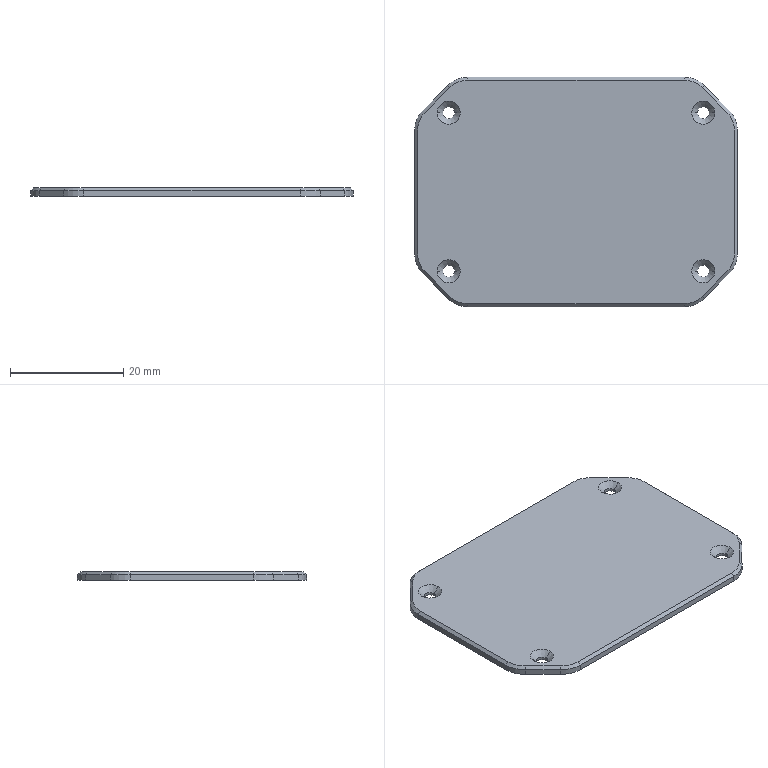NC program | NX | posted with a generic post | part box 57 x 40.5 x 1.5 mm
Lines 1 to 1491 of 7802:
N10 G17 G21 G94 G90
(PLANAR_PROFILE , TOOL : D4)
N12 T01 M6
N14 G54
N16 G17 G0 G90 X2.1 Y31.609 S6500 M3
N18 G43 Z20. H1
N20 Z0.1
N22 G94 G1 Y8.668 Z0.06 F1200.
N24 X1.827 Y7.266 Z0.057
N26 X1.281 Y5.947 Z0.055
N28 X0.482 Y4.763 Z0.052
N30 X-4.763 Y-0.482 Z0.04
N32 X-5.947 Y-1.281 Z0.037
N34 X-7.266 Y-1.827 Z0.035
N36 X-8.668 Y-2.1 Z0.032
N38 X-48.332 Z-0.037
N40 X-49.734 Y-1.827 Z-0.04
N42 X-51.053 Y-1.281 Z-0.042
N44 X-52.237 Y-0.482 Z-0.045
N46 X-57.482 Y4.763 Z-0.058
N48 X-58.281 Y5.947 Z-0.06
N50 X-58.827 Y7.266 Z-0.063
N52 X-59.1 Y8.668 Z-0.065
N54 Y31.832 Z-0.106
N56 X-58.827 Y33.234 Z-0.108
N58 X-58.281 Y34.553 Z-0.11
N60 X-57.482 Y35.737 Z-0.113
N62 X-52.237 Y40.982 Z-0.126
N64 X-51.053 Y41.781 Z-0.128
N66 X-49.734 Y42.327 Z-0.131
N68 X-48.332 Y42.6 Z-0.133
N70 X-8.668 Z-0.203
N72 X-7.266 Y42.327 Z-0.205
N74 X-5.947 Y41.781 Z-0.208
N76 X-4.763 Y40.982 Z-0.21
N78 X0.482 Y35.737 Z-0.223
N80 X1.281 Y34.553 Z-0.226
N82 X1.827 Y33.234 Z-0.228
N84 X2.1 Y31.832 Z-0.231
N86 Y8.668 Z-0.271
N88 X1.827 Y7.266 Z-0.273
N90 X1.281 Y5.947 Z-0.276
N92 X0.482 Y4.763 Z-0.278
N94 X-4.763 Y-0.482 Z-0.291
N96 X-5.947 Y-1.281 Z-0.294
N98 X-7.266 Y-1.827 Z-0.296
N100 X-8.668 Y-2.1 Z-0.299
N102 X-9.321 Z-0.3
N104 X-47.679 F2000.
N106 G2 X-52.699 Y-0.02 R7.1
N108 G1 X-57.02 Y4.301
N110 G2 X-59.1 Y9.321 R7.1
N112 G1 Y31.179
N114 G2 X-57.02 Y36.199 R7.1
N116 G1 X-52.699 Y40.52
N118 G2 X-47.679 Y42.6 R7.1
N120 G1 X-9.321
N122 G2 X-4.301 Y40.52 R7.1
N124 G1 X0.02 Y36.199
N126 G2 X2.1 Y31.179 R7.1
N128 G1 Y9.321
N130 G2 X0.02 Y4.301 R7.1
N132 G1 X-4.301 Y-0.02
N134 G2 X-9.321 Y-2.1 R7.1
N136 G1 Z-0.2
N138 G0 Z20.
N140 X2.1 Y31.609
N142 Z-0.2
N144 G1 Y8.668 Z-0.24 F1200.
N146 X1.827 Y7.266 Z-0.243
N148 X1.281 Y5.947 Z-0.245
N150 X0.482 Y4.763 Z-0.248
N152 X-4.763 Y-0.482 Z-0.26
N154 X-5.947 Y-1.281 Z-0.263
N156 X-7.266 Y-1.827 Z-0.265
N158 X-8.668 Y-2.1 Z-0.268
N160 X-48.332 Z-0.337
N162 X-49.734 Y-1.827 Z-0.34
N164 X-51.053 Y-1.281 Z-0.342
N166 X-52.237 Y-0.482 Z-0.345
N168 X-57.482 Y4.763 Z-0.358
N170 X-58.281 Y5.947 Z-0.36
N172 X-58.827 Y7.266 Z-0.363
N174 X-59.1 Y8.668 Z-0.365
N176 Y31.832 Z-0.406
N178 X-58.827 Y33.234 Z-0.408
N180 X-58.281 Y34.553 Z-0.41
N182 X-57.482 Y35.737 Z-0.413
N184 X-52.237 Y40.982 Z-0.426
N186 X-51.053 Y41.781 Z-0.428
N188 X-49.734 Y42.327 Z-0.431
N190 X-48.332 Y42.6 Z-0.433
N192 X-8.668 Z-0.503
N194 X-7.266 Y42.327 Z-0.505
N196 X-5.947 Y41.781 Z-0.508
N198 X-4.763 Y40.982 Z-0.51
N200 X0.482 Y35.737 Z-0.523
N202 X1.281 Y34.553 Z-0.526
N204 X1.827 Y33.234 Z-0.528
N206 X2.1 Y31.832 Z-0.531
N208 Y8.668 Z-0.571
N210 X1.827 Y7.266 Z-0.573
N212 X1.281 Y5.947 Z-0.576
N214 X0.482 Y4.763 Z-0.578
N216 X-4.763 Y-0.482 Z-0.591
N218 X-5.947 Y-1.281 Z-0.594
N220 X-7.266 Y-1.827 Z-0.596
N222 X-8.668 Y-2.1 Z-0.599
N224 X-9.321 Z-0.6
N226 X-47.679 F2000.
N228 G2 X-52.699 Y-0.02 R7.1
N230 G1 X-57.02 Y4.301
N232 G2 X-59.1 Y9.321 R7.1
N234 G1 Y31.179
N236 G2 X-57.02 Y36.199 R7.1
N238 G1 X-52.699 Y40.52
N240 G2 X-47.679 Y42.6 R7.1
N242 G1 X-9.321
N244 G2 X-4.301 Y40.52 R7.1
N246 G1 X0.02 Y36.199
N248 G2 X2.1 Y31.179 R7.1
N250 G1 Y9.321
N252 G2 X0.02 Y4.301 R7.1
N254 G1 X-4.301 Y-0.02
N256 G2 X-9.321 Y-2.1 R7.1
N258 G1 Z-0.5
N260 G0 Z20.
N262 X2.1 Y31.609
N264 Z-0.5
N266 G1 Y8.668 Z-0.54 F1200.
N268 X1.827 Y7.266 Z-0.543
N270 X1.281 Y5.947 Z-0.545
N272 X0.482 Y4.763 Z-0.548
N274 X-4.763 Y-0.482 Z-0.56
N276 X-5.947 Y-1.281 Z-0.563
N278 X-7.266 Y-1.827 Z-0.565
N280 X-8.668 Y-2.1 Z-0.568
N282 X-48.332 Z-0.637
N284 X-49.734 Y-1.827 Z-0.64
N286 X-51.053 Y-1.281 Z-0.642
N288 X-52.237 Y-0.482 Z-0.645
N290 X-57.482 Y4.763 Z-0.658
N292 X-58.281 Y5.947 Z-0.66
N294 X-58.827 Y7.266 Z-0.663
N296 X-59.1 Y8.668 Z-0.665
N298 Y31.832 Z-0.706
N300 X-58.827 Y33.234 Z-0.708
N302 X-58.281 Y34.553 Z-0.71
N304 X-57.482 Y35.737 Z-0.713
N306 X-52.237 Y40.982 Z-0.726
N308 X-51.053 Y41.781 Z-0.728
N310 X-49.734 Y42.327 Z-0.731
N312 X-48.332 Y42.6 Z-0.733
N314 X-8.668 Z-0.803
N316 X-7.266 Y42.327 Z-0.805
N318 X-5.947 Y41.781 Z-0.808
N320 X-4.763 Y40.982 Z-0.81
N322 X0.482 Y35.737 Z-0.823
N324 X1.281 Y34.553 Z-0.826
N326 X1.827 Y33.234 Z-0.828
N328 X2.1 Y31.832 Z-0.831
N330 Y8.668 Z-0.871
N332 X1.827 Y7.266 Z-0.873
N334 X1.281 Y5.947 Z-0.876
N336 X0.482 Y4.763 Z-0.878
N338 X-4.763 Y-0.482 Z-0.891
N340 X-5.947 Y-1.281 Z-0.894
N342 X-7.266 Y-1.827 Z-0.896
N344 X-8.668 Y-2.1 Z-0.899
N346 X-9.321 Z-0.9
N348 X-47.679 F2000.
N350 G2 X-52.699 Y-0.02 R7.1
N352 G1 X-57.02 Y4.301
N354 G2 X-59.1 Y9.321 R7.1
N356 G1 Y31.179
N358 G2 X-57.02 Y36.199 R7.1
N360 G1 X-52.699 Y40.52
N362 G2 X-47.679 Y42.6 R7.1
N364 G1 X-9.321
N366 G2 X-4.301 Y40.52 R7.1
N368 G1 X0.02 Y36.199
N370 G2 X2.1 Y31.179 R7.1
N372 G1 Y9.321
N374 G2 X0.02 Y4.301 R7.1
N376 G1 X-4.301 Y-0.02
N378 G2 X-9.321 Y-2.1 R7.1
N380 G1 Z-0.8
N382 G0 Z20.
N384 X2.1 Y31.609
N386 Z-0.8
N388 G1 Y8.668 Z-0.84 F1200.
N390 X1.827 Y7.266 Z-0.843
N392 X1.281 Y5.947 Z-0.845
N394 X0.482 Y4.763 Z-0.848
N396 X-4.763 Y-0.482 Z-0.86
N398 X-5.947 Y-1.281 Z-0.863
N400 X-7.266 Y-1.827 Z-0.865
N402 X-8.668 Y-2.1 Z-0.868
N404 X-48.332 Z-0.937
N406 X-49.734 Y-1.827 Z-0.94
N408 X-51.053 Y-1.281 Z-0.942
N410 X-52.237 Y-0.482 Z-0.945
N412 X-57.482 Y4.763 Z-0.958
N414 X-58.281 Y5.947 Z-0.96
N416 X-58.827 Y7.266 Z-0.963
N418 X-59.1 Y8.668 Z-0.965
N420 Y31.832 Z-1.006
N422 X-58.827 Y33.234 Z-1.008
N424 X-58.281 Y34.553 Z-1.01
N426 X-57.482 Y35.737 Z-1.013
N428 X-52.237 Y40.982 Z-1.026
N430 X-51.053 Y41.781 Z-1.028
N432 X-49.734 Y42.327 Z-1.031
N434 X-48.332 Y42.6 Z-1.033
N436 X-8.668 Z-1.103
N438 X-7.266 Y42.327 Z-1.105
N440 X-5.947 Y41.781 Z-1.108
N442 X-4.763 Y40.982 Z-1.11
N444 X0.482 Y35.737 Z-1.123
N446 X1.281 Y34.553 Z-1.126
N448 X1.827 Y33.234 Z-1.128
N450 X2.1 Y31.832 Z-1.131
N452 Y8.668 Z-1.171
N454 X1.827 Y7.266 Z-1.173
N456 X1.281 Y5.947 Z-1.176
N458 X0.482 Y4.763 Z-1.178
N460 X-4.763 Y-0.482 Z-1.191
N462 X-5.947 Y-1.281 Z-1.194
N464 X-7.266 Y-1.827 Z-1.196
N466 X-8.668 Y-2.1 Z-1.199
N468 X-9.321 Z-1.2
N470 X-47.679 F2000.
N472 G2 X-52.699 Y-0.02 R7.1
N474 G1 X-57.02 Y4.301
N476 G2 X-59.1 Y9.321 R7.1
N478 G1 Y31.179
N480 G2 X-57.02 Y36.199 R7.1
N482 G1 X-52.699 Y40.52
N484 G2 X-47.679 Y42.6 R7.1
N486 G1 X-9.321
N488 G2 X-4.301 Y40.52 R7.1
N490 G1 X0.02 Y36.199
N492 G2 X2.1 Y31.179 R7.1
N494 G1 Y9.321
N496 G2 X0.02 Y4.301 R7.1
N498 G1 X-4.301 Y-0.02
N500 G2 X-9.321 Y-2.1 R7.1
N502 G1 Z-1.1
N504 G0 Z20.
N506 X2.1 Y31.609
N508 Z-1.1
N510 G1 Y8.668 Z-1.14 F1200.
N512 X1.827 Y7.266 Z-1.143
N514 X1.281 Y5.947 Z-1.145
N516 X0.482 Y4.763 Z-1.148
N518 X-4.763 Y-0.482 Z-1.16
N520 X-5.947 Y-1.281 Z-1.163
N522 X-7.266 Y-1.827 Z-1.165
N524 X-8.668 Y-2.1 Z-1.168
N526 X-48.332 Z-1.237
N528 X-49.734 Y-1.827 Z-1.24
N530 X-51.053 Y-1.281 Z-1.242
N532 X-52.237 Y-0.482 Z-1.245
N534 X-57.482 Y4.763 Z-1.258
N536 X-58.281 Y5.947 Z-1.26
N538 X-58.827 Y7.266 Z-1.263
N540 X-59.1 Y8.668 Z-1.265
N542 Y31.832 Z-1.306
N544 X-58.827 Y33.234 Z-1.308
N546 X-58.281 Y34.553 Z-1.31
N548 X-57.482 Y35.737 Z-1.313
N550 X-52.237 Y40.982 Z-1.326
N552 X-51.053 Y41.781 Z-1.328
N554 X-49.734 Y42.327 Z-1.331
N556 X-48.332 Y42.6 Z-1.333
N558 X-8.668 Z-1.403
N560 X-7.266 Y42.327 Z-1.405
N562 X-5.947 Y41.781 Z-1.408
N564 X-4.763 Y40.982 Z-1.41
N566 X0.482 Y35.737 Z-1.423
N568 X1.281 Y34.553 Z-1.426
N570 X1.827 Y33.234 Z-1.428
N572 X2.1 Y31.832 Z-1.431
N574 Y8.668 Z-1.471
N576 X1.827 Y7.266 Z-1.473
N578 X1.281 Y5.947 Z-1.476
N580 X0.482 Y4.763 Z-1.478
N582 X-4.763 Y-0.482 Z-1.491
N584 X-5.947 Y-1.281 Z-1.494
N586 X-7.266 Y-1.827 Z-1.496
N588 X-8.668 Y-2.1 Z-1.499
N590 X-9.321 Z-1.5
N592 X-47.679 F2000.
N594 G2 X-52.699 Y-0.02 R7.1
N596 G1 X-57.02 Y4.301
N598 G2 X-59.1 Y9.321 R7.1
N600 G1 Y31.179
N602 G2 X-57.02 Y36.199 R7.1
N604 G1 X-52.699 Y40.52
N606 G2 X-47.679 Y42.6 R7.1
N608 G1 X-9.321
N610 G2 X-4.301 Y40.52 R7.1
N612 G1 X0.02 Y36.199
N614 G2 X2.1 Y31.179 R7.1
N616 G1 Y9.321
N618 G2 X0.02 Y4.301 R7.1
N620 G1 X-4.301 Y-0.02
N622 G2 X-9.321 Y-2.1 R7.1
N624 G1 Z-1.4
N626 G0 Z20.
(PLANAR_PROFILE_COPY , TOOL : D4)
N628 X-9.221
N630 Z1.5
N632 G1 Z-1.5 F800.
N634 X-9.232 Y-2.049
N636 X-9.27 Y-2.011
N638 X-9.321 Y-2.
N640 X-47.679
N642 G2 X-52.629 Y0.05 R7.
N644 G1 X-56.95 Y4.371
N646 G2 X-59. Y9.321 R7.
N648 G1 Y31.179
N650 G2 X-56.95 Y36.129 R7.
N652 G1 X-52.629 Y40.45
N654 G2 X-47.679 Y42.5 R7.
N656 G1 X-9.321
N658 G2 X-4.371 Y40.45 R7.
N660 G1 X-0.05 Y36.129
N662 G2 X2. Y31.179 R7.
N664 G1 Y9.321
N666 G2 X-0.05 Y4.371 R7.
N668 G1 X-4.371 Y0.05
N670 G2 X-9.321 Y-2. R7.
N672 G1 X-9.373 Y-2.011
N674 X-9.41 Y-2.049
N676 X-9.421 Y-2.1
N678 Z1.5
N680 G0 Z20.
N682 M5
(PLANAR_PROFILE_COPY_COPY , TOOL : D3倒角)
N684 T02 M6
N686 G54
N688 G17 G0 G90 X-7.321 Y-2.6 S4500 M3
N690 G43 Z20. H2
N692 Z2.
N694 G94 G1 Z-1. F800.
N696 G3 X-9.321 Y-0.6 R2.
N698 G1 X-47.679
N700 G2 X-51.639 Y1.04 R5.6
N702 G1 X-55.96 Y5.361
N704 G2 X-57.6 Y9.321 R5.6
N706 G1 Y31.179
N708 G2 X-55.96 Y35.139 R5.6
N710 G1 X-51.639 Y39.46
N712 G2 X-47.679 Y41.1 R5.6
N714 G1 X-9.321
N716 G2 X-5.361 Y39.46 R5.6
N718 G1 X-1.04 Y35.139
N720 G2 X0.6 Y31.179 R5.6
N722 G1 Y9.321
N724 G2 X-1.04 Y5.361 R5.6
N726 G1 X-5.361 Y1.04
N728 G2 X-9.321 Y-0.6 R5.6
N730 G3 X-11.321 Y-2.6 R2.
N732 G1 Z2.
N734 G0 Z20.
N736 M5
(PLANAR_PROFILE_COPY_1 , TOOL : D4)
N738 T01 M6
N740 G54
N742 G17 G0 G90 X-59.9 Y31.609 S6500 M3
N744 G43 Z20. H1
N746 Z0.1
N748 G94 G1 Y8.668 Z0.06 F1200.
N750 X-60.173 Y7.266 Z0.057
N752 X-60.719 Y5.947 Z0.055
N754 X-61.518 Y4.763 Z0.052
N756 X-66.763 Y-0.482 Z0.04
N758 X-67.947 Y-1.281 Z0.037
N760 X-69.266 Y-1.827 Z0.035
N762 X-70.668 Y-2.1 Z0.032
N764 X-110.332 Z-0.037
N766 X-111.734 Y-1.827 Z-0.04
N768 X-113.053 Y-1.281 Z-0.042
N770 X-114.237 Y-0.482 Z-0.045
N772 X-119.482 Y4.763 Z-0.058
N774 X-120.281 Y5.947 Z-0.06
N776 X-120.827 Y7.266 Z-0.063
N778 X-121.1 Y8.668 Z-0.065
N780 Y31.832 Z-0.106
N782 X-120.827 Y33.234 Z-0.108
N784 X-120.281 Y34.553 Z-0.11
N786 X-119.482 Y35.737 Z-0.113
N788 X-114.237 Y40.982 Z-0.126
N790 X-113.053 Y41.781 Z-0.128
N792 X-111.734 Y42.327 Z-0.131
N794 X-110.332 Y42.6 Z-0.133
N796 X-70.668 Z-0.203
N798 X-69.266 Y42.327 Z-0.205
N800 X-67.947 Y41.781 Z-0.208
N802 X-66.763 Y40.982 Z-0.21
N804 X-61.518 Y35.737 Z-0.223
N806 X-60.719 Y34.553 Z-0.226
N808 X-60.173 Y33.234 Z-0.228
N810 X-59.9 Y31.832 Z-0.231
N812 Y8.668 Z-0.271
N814 X-60.173 Y7.266 Z-0.273
N816 X-60.719 Y5.947 Z-0.276
N818 X-61.518 Y4.763 Z-0.278
N820 X-66.763 Y-0.482 Z-0.291
N822 X-67.947 Y-1.281 Z-0.294
N824 X-69.266 Y-1.827 Z-0.296
N826 X-70.668 Y-2.1 Z-0.299
N828 X-71.321 Z-0.3
N830 X-109.679 F2000.
N832 G2 X-114.699 Y-0.02 R7.1
N834 G1 X-119.02 Y4.301
N836 G2 X-121.1 Y9.321 R7.1
N838 G1 Y31.179
N840 G2 X-119.02 Y36.199 R7.1
N842 G1 X-114.699 Y40.52
N844 G2 X-109.679 Y42.6 R7.1
N846 G1 X-71.321
N848 G2 X-66.301 Y40.52 R7.1
N850 G1 X-61.98 Y36.199
N852 G2 X-59.9 Y31.179 R7.1
N854 G1 Y9.321
N856 G2 X-61.98 Y4.301 R7.1
N858 G1 X-66.301 Y-0.02
N860 G2 X-71.321 Y-2.1 R7.1
N862 G1 Z-0.2
N864 G0 Z20.
N866 X-59.9 Y31.609
N868 Z-0.2
N870 G1 Y8.668 Z-0.24 F1200.
N872 X-60.173 Y7.266 Z-0.243
N874 X-60.719 Y5.947 Z-0.245
N876 X-61.518 Y4.763 Z-0.248
N878 X-66.763 Y-0.482 Z-0.26
N880 X-67.947 Y-1.281 Z-0.263
N882 X-69.266 Y-1.827 Z-0.265
N884 X-70.668 Y-2.1 Z-0.268
N886 X-110.332 Z-0.337
N888 X-111.734 Y-1.827 Z-0.34
N890 X-113.053 Y-1.281 Z-0.342
N892 X-114.237 Y-0.482 Z-0.345
N894 X-119.482 Y4.763 Z-0.358
N896 X-120.281 Y5.947 Z-0.36
N898 X-120.827 Y7.266 Z-0.363
N900 X-121.1 Y8.668 Z-0.365
N902 Y31.832 Z-0.406
N904 X-120.827 Y33.234 Z-0.408
N906 X-120.281 Y34.553 Z-0.41
N908 X-119.482 Y35.737 Z-0.413
N910 X-114.237 Y40.982 Z-0.426
N912 X-113.053 Y41.781 Z-0.428
N914 X-111.734 Y42.327 Z-0.431
N916 X-110.332 Y42.6 Z-0.433
N918 X-70.668 Z-0.503
N920 X-69.266 Y42.327 Z-0.505
N922 X-67.947 Y41.781 Z-0.508
N924 X-66.763 Y40.982 Z-0.51
N926 X-61.518 Y35.737 Z-0.523
N928 X-60.719 Y34.553 Z-0.526
N930 X-60.173 Y33.234 Z-0.528
N932 X-59.9 Y31.832 Z-0.531
N934 Y8.668 Z-0.571
N936 X-60.173 Y7.266 Z-0.573
N938 X-60.719 Y5.947 Z-0.576
N940 X-61.518 Y4.763 Z-0.578
N942 X-66.763 Y-0.482 Z-0.591
N944 X-67.947 Y-1.281 Z-0.594
N946 X-69.266 Y-1.827 Z-0.596
N948 X-70.668 Y-2.1 Z-0.599
N950 X-71.321 Z-0.6
N952 X-109.679 F2000.
N954 G2 X-114.699 Y-0.02 R7.1
N956 G1 X-119.02 Y4.301
N958 G2 X-121.1 Y9.321 R7.1
N960 G1 Y31.179
N962 G2 X-119.02 Y36.199 R7.1
N964 G1 X-114.699 Y40.52
N966 G2 X-109.679 Y42.6 R7.1
N968 G1 X-71.321
N970 G2 X-66.301 Y40.52 R7.1
N972 G1 X-61.98 Y36.199
N974 G2 X-59.9 Y31.179 R7.1
N976 G1 Y9.321
N978 G2 X-61.98 Y4.301 R7.1
N980 G1 X-66.301 Y-0.02
N982 G2 X-71.321 Y-2.1 R7.1
N984 G1 Z-0.5
N986 G0 Z20.
N988 X-59.9 Y31.609
N990 Z-0.5
N992 G1 Y8.668 Z-0.54 F1200.
N994 X-60.173 Y7.266 Z-0.543
N996 X-60.719 Y5.947 Z-0.545
N998 X-61.518 Y4.763 Z-0.548
N1000 X-66.763 Y-0.482 Z-0.56
N1002 X-67.947 Y-1.281 Z-0.563
N1004 X-69.266 Y-1.827 Z-0.565
N1006 X-70.668 Y-2.1 Z-0.568
N1008 X-110.332 Z-0.637
N1010 X-111.734 Y-1.827 Z-0.64
N1012 X-113.053 Y-1.281 Z-0.642
N1014 X-114.237 Y-0.482 Z-0.645
N1016 X-119.482 Y4.763 Z-0.658
N1018 X-120.281 Y5.947 Z-0.66
N1020 X-120.827 Y7.266 Z-0.663
N1022 X-121.1 Y8.668 Z-0.665
N1024 Y31.832 Z-0.706
N1026 X-120.827 Y33.234 Z-0.708
N1028 X-120.281 Y34.553 Z-0.71
N1030 X-119.482 Y35.737 Z-0.713
N1032 X-114.237 Y40.982 Z-0.726
N1034 X-113.053 Y41.781 Z-0.728
N1036 X-111.734 Y42.327 Z-0.731
N1038 X-110.332 Y42.6 Z-0.733
N1040 X-70.668 Z-0.803
N1042 X-69.266 Y42.327 Z-0.805
N1044 X-67.947 Y41.781 Z-0.808
N1046 X-66.763 Y40.982 Z-0.81
N1048 X-61.518 Y35.737 Z-0.823
N1050 X-60.719 Y34.553 Z-0.826
N1052 X-60.173 Y33.234 Z-0.828
N1054 X-59.9 Y31.832 Z-0.831
N1056 Y8.668 Z-0.871
N1058 X-60.173 Y7.266 Z-0.873
N1060 X-60.719 Y5.947 Z-0.876
N1062 X-61.518 Y4.763 Z-0.878
N1064 X-66.763 Y-0.482 Z-0.891
N1066 X-67.947 Y-1.281 Z-0.894
N1068 X-69.266 Y-1.827 Z-0.896
N1070 X-70.668 Y-2.1 Z-0.899
N1072 X-71.321 Z-0.9
N1074 X-109.679 F2000.
N1076 G2 X-114.699 Y-0.02 R7.1
N1078 G1 X-119.02 Y4.301
N1080 G2 X-121.1 Y9.321 R7.1
N1082 G1 Y31.179
N1084 G2 X-119.02 Y36.199 R7.1
N1086 G1 X-114.699 Y40.52
N1088 G2 X-109.679 Y42.6 R7.1
N1090 G1 X-71.321
N1092 G2 X-66.301 Y40.52 R7.1
N1094 G1 X-61.98 Y36.199
N1096 G2 X-59.9 Y31.179 R7.1
N1098 G1 Y9.321
N1100 G2 X-61.98 Y4.301 R7.1
N1102 G1 X-66.301 Y-0.02
N1104 G2 X-71.321 Y-2.1 R7.1
N1106 G1 Z-0.8
N1108 G0 Z20.
N1110 X-59.9 Y31.609
N1112 Z-0.8
N1114 G1 Y8.668 Z-0.84 F1200.
N1116 X-60.173 Y7.266 Z-0.843
N1118 X-60.719 Y5.947 Z-0.845
N1120 X-61.518 Y4.763 Z-0.848
N1122 X-66.763 Y-0.482 Z-0.86
N1124 X-67.947 Y-1.281 Z-0.863
N1126 X-69.266 Y-1.827 Z-0.865
N1128 X-70.668 Y-2.1 Z-0.868
N1130 X-110.332 Z-0.937
N1132 X-111.734 Y-1.827 Z-0.94
N1134 X-113.053 Y-1.281 Z-0.942
N1136 X-114.237 Y-0.482 Z-0.945
N1138 X-119.482 Y4.763 Z-0.958
N1140 X-120.281 Y5.947 Z-0.96
N1142 X-120.827 Y7.266 Z-0.963
N1144 X-121.1 Y8.668 Z-0.965
N1146 Y31.832 Z-1.006
N1148 X-120.827 Y33.234 Z-1.008
N1150 X-120.281 Y34.553 Z-1.01
N1152 X-119.482 Y35.737 Z-1.013
N1154 X-114.237 Y40.982 Z-1.026
N1156 X-113.053 Y41.781 Z-1.028
N1158 X-111.734 Y42.327 Z-1.031
N1160 X-110.332 Y42.6 Z-1.033
N1162 X-70.668 Z-1.103
N1164 X-69.266 Y42.327 Z-1.105
N1166 X-67.947 Y41.781 Z-1.108
N1168 X-66.763 Y40.982 Z-1.11
N1170 X-61.518 Y35.737 Z-1.123
N1172 X-60.719 Y34.553 Z-1.126
N1174 X-60.173 Y33.234 Z-1.128
N1176 X-59.9 Y31.832 Z-1.131
N1178 Y8.668 Z-1.171
N1180 X-60.173 Y7.266 Z-1.173
N1182 X-60.719 Y5.947 Z-1.176
N1184 X-61.518 Y4.763 Z-1.178
N1186 X-66.763 Y-0.482 Z-1.191
N1188 X-67.947 Y-1.281 Z-1.194
N1190 X-69.266 Y-1.827 Z-1.196
N1192 X-70.668 Y-2.1 Z-1.199
N1194 X-71.321 Z-1.2
N1196 X-109.679 F2000.
N1198 G2 X-114.699 Y-0.02 R7.1
N1200 G1 X-119.02 Y4.301
N1202 G2 X-121.1 Y9.321 R7.1
N1204 G1 Y31.179
N1206 G2 X-119.02 Y36.199 R7.1
N1208 G1 X-114.699 Y40.52
N1210 G2 X-109.679 Y42.6 R7.1
N1212 G1 X-71.321
N1214 G2 X-66.301 Y40.52 R7.1
N1216 G1 X-61.98 Y36.199
N1218 G2 X-59.9 Y31.179 R7.1
N1220 G1 Y9.321
N1222 G2 X-61.98 Y4.301 R7.1
N1224 G1 X-66.301 Y-0.02
N1226 G2 X-71.321 Y-2.1 R7.1
N1228 G1 Z-1.1
N1230 G0 Z20.
N1232 X-59.9 Y31.609
N1234 Z-1.1
N1236 G1 Y8.668 Z-1.14 F1200.
N1238 X-60.173 Y7.266 Z-1.143
N1240 X-60.719 Y5.947 Z-1.145
N1242 X-61.518 Y4.763 Z-1.148
N1244 X-66.763 Y-0.482 Z-1.16
N1246 X-67.947 Y-1.281 Z-1.163
N1248 X-69.266 Y-1.827 Z-1.165
N1250 X-70.668 Y-2.1 Z-1.168
N1252 X-110.332 Z-1.237
N1254 X-111.734 Y-1.827 Z-1.24
N1256 X-113.053 Y-1.281 Z-1.242
N1258 X-114.237 Y-0.482 Z-1.245
N1260 X-119.482 Y4.763 Z-1.258
N1262 X-120.281 Y5.947 Z-1.26
N1264 X-120.827 Y7.266 Z-1.263
N1266 X-121.1 Y8.668 Z-1.265
N1268 Y31.832 Z-1.306
N1270 X-120.827 Y33.234 Z-1.308
N1272 X-120.281 Y34.553 Z-1.31
N1274 X-119.482 Y35.737 Z-1.313
N1276 X-114.237 Y40.982 Z-1.326
N1278 X-113.053 Y41.781 Z-1.328
N1280 X-111.734 Y42.327 Z-1.331
N1282 X-110.332 Y42.6 Z-1.333
N1284 X-70.668 Z-1.403
N1286 X-69.266 Y42.327 Z-1.405
N1288 X-67.947 Y41.781 Z-1.408
N1290 X-66.763 Y40.982 Z-1.41
N1292 X-61.518 Y35.737 Z-1.423
N1294 X-60.719 Y34.553 Z-1.426
N1296 X-60.173 Y33.234 Z-1.428
N1298 X-59.9 Y31.832 Z-1.431
N1300 Y8.668 Z-1.471
N1302 X-60.173 Y7.266 Z-1.473
N1304 X-60.719 Y5.947 Z-1.476
N1306 X-61.518 Y4.763 Z-1.478
N1308 X-66.763 Y-0.482 Z-1.491
N1310 X-67.947 Y-1.281 Z-1.494
N1312 X-69.266 Y-1.827 Z-1.496
N1314 X-70.668 Y-2.1 Z-1.499
N1316 X-71.321 Z-1.5
N1318 X-109.679 F2000.
N1320 G2 X-114.699 Y-0.02 R7.1
N1322 G1 X-119.02 Y4.301
N1324 G2 X-121.1 Y9.321 R7.1
N1326 G1 Y31.179
N1328 G2 X-119.02 Y36.199 R7.1
N1330 G1 X-114.699 Y40.52
N1332 G2 X-109.679 Y42.6 R7.1
N1334 G1 X-71.321
N1336 G2 X-66.301 Y40.52 R7.1
N1338 G1 X-61.98 Y36.199
N1340 G2 X-59.9 Y31.179 R7.1
N1342 G1 Y9.321
N1344 G2 X-61.98 Y4.301 R7.1
N1346 G1 X-66.301 Y-0.02
N1348 G2 X-71.321 Y-2.1 R7.1
N1350 G1 Z-1.4
N1352 G0 Z20.
(PLANAR_PROFILE_COPY_COPY_1 , TOOL : D4)
N1354 X-71.221
N1356 Z1.5
N1358 G1 Z-1.5 F800.
N1360 X-71.232 Y-2.049
N1362 X-71.27 Y-2.011
N1364 X-71.321 Y-2.
N1366 X-109.679
N1368 G2 X-114.629 Y0.05 R7.
N1370 G1 X-118.95 Y4.371
N1372 G2 X-121. Y9.321 R7.
N1374 G1 Y31.179
N1376 G2 X-118.95 Y36.129 R7.
N1378 G1 X-114.629 Y40.45
N1380 G2 X-109.679 Y42.5 R7.
N1382 G1 X-71.321
N1384 G2 X-66.371 Y40.45 R7.
N1386 G1 X-62.05 Y36.129
N1388 G2 X-60. Y31.179 R7.
N1390 G1 Y9.321
N1392 G2 X-62.05 Y4.371 R7.
N1394 G1 X-66.371 Y0.05
N1396 G2 X-71.321 Y-2. R7.
N1398 G1 X-71.373 Y-2.011
N1400 X-71.41 Y-2.049
N1402 X-71.421 Y-2.1
N1404 Z1.5
N1406 G0 Z20.
N1408 M5
(PLANAR_PROFILE_COPY_COPY_COPY , TOOL : D3倒角)
N1410 T02 M6
N1412 G54
N1414 G17 G0 G90 X-69.321 Y-2.6 S4500 M3
N1416 G43 Z20. H2
N1418 Z2.
N1420 G94 G1 Z-1. F800.
N1422 G3 X-71.321 Y-0.6 R2.
N1424 G1 X-109.679
N1426 G2 X-113.639 Y1.04 R5.6
N1428 G1 X-117.96 Y5.361
N1430 G2 X-119.6 Y9.321 R5.6
N1432 G1 Y31.179
N1434 G2 X-117.96 Y35.139 R5.6
N1436 G1 X-113.639 Y39.46
N1438 G2 X-109.679 Y41.1 R5.6
N1440 G1 X-71.321
N1442 G2 X-67.361 Y39.46 R5.6
N1444 G1 X-63.04 Y35.139
N1446 G2 X-61.4 Y31.179 R5.6
N1448 G1 Y9.321
N1450 G2 X-63.04 Y5.361 R5.6
N1452 G1 X-67.361 Y1.04
N1454 G2 X-71.321 Y-0.6 R5.6
N1456 G3 X-73.321 Y-2.6 R2.
N1458 G1 Z2.
N1460 G0 Z20.
N1462 M5
(PLANAR_PROFILE_COPY_2 , TOOL : D4)
N1464 T01 M6
N1466 G54
N1468 G17 G0 G90 X-121.9 Y31.609 S6500 M3
N1470 G43 Z20. H1
N1472 Z0.1
N1474 G94 G1 Y8.668 Z0.06 F1200.
N1476 X-122.173 Y7.266 Z0.057
N1478 X-122.719 Y5.947 Z0.055
N1480 X-123.518 Y4.763 Z0.052
N1482 X-128.763 Y-0.482 Z0.04
N1484 X-129.947 Y-1.281 Z0.037
N1486 X-131.266 Y-1.827 Z0.035
N1488 X-132.668 Y-2.1 Z0.032
N1490 X-172.332 Z-0.037
N1492 X-173.734 Y-1.827 Z-0.04
N1494 X-175.053 Y-1.281 Z-0.042
N1496 X-176.237 Y-0.482 Z-0.045
N1498 X-181.482 Y4.763 Z-0.058
N1500 X-182.281 Y5.947 Z-0.06
N1502 X-182.827 Y7.266 Z-0.063
N1504 X-183.1 Y8.668 Z-0.065
N1506 Y31.832 Z-0.106
N1508 X-182.827 Y33.234 Z-0.108
N1510 X-182.281 Y34.553 Z-0.11
N1512 X-181.482 Y35.737 Z-0.113
N1514 X-176.237 Y40.982 Z-0.126
N1516 X-175.053 Y41.781 Z-0.128
N1518 X-173.734 Y42.327 Z-0.131
N1520 X-172.332 Y42.6 Z-0.133
N1522 X-132.668 Z-0.203
N1524 X-131.266 Y42.327 Z-0.205
N1526 X-129.947 Y41.781 Z-0.208
N1528 X-128.763 Y40.982 Z-0.21
N1530 X-123.518 Y35.737 Z-0.223
N1532 X-122.719 Y34.553 Z-0.226
N1534 X-122.173 Y33.234 Z-0.228
N1536 X-121.9 Y31.832 Z-0.231
N1538 Y8.668 Z-0.271
N1540 X-122.173 Y7.266 Z-0.273
N1542 X-122.719 Y5.947 Z-0.276
N1544 X-123.518 Y4.763 Z-0.278
N1546 X-128.763 Y-0.482 Z-0.291
N1548 X-129.947 Y-1.281 Z-0.294
N1550 X-131.266 Y-1.827 Z-0.296
N1552 X-132.668 Y-2.1 Z-0.299
N1554 X-133.321 Z-0.3
N1556 X-171.679 F2000.
N1558 G2 X-176.699 Y-0.02 R7.1
N1560 G1 X-181.02 Y4.301
N1562 G2 X-183.1 Y9.321 R7.1
N1564 G1 Y31.179
N1566 G2 X-181.02 Y36.199 R7.1
N1568 G1 X-176.699 Y40.52
N1570 G2 X-171.679 Y42.6 R7.1
N1572 G1 X-133.321
N1574 G2 X-128.301 Y40.52 R7.1
N1576 G1 X-123.98 Y36.199
N1578 G2 X-121.9 Y31.179 R7.1
N1580 G1 Y9.321
N1582 G2 X-123.98 Y4.301 R7.1
N1584 G1 X-128.301 Y-0.02
N1586 G2 X-133.321 Y-2.1 R7.1
N1588 G1 Z-0.2
N1590 G0 Z20.
N1592 X-121.9 Y31.609
N1594 Z-0.2
N1596 G1 Y8.668 Z-0.24 F1200.
N1598 X-122.173 Y7.266 Z-0.243
N1600 X-122.719 Y5.947 Z-0.245
N1602 X-123.518 Y4.763 Z-0.248
N1604 X-128.763 Y-0.482 Z-0.26
N1606 X-129.947 Y-1.281 Z-0.263
N1608 X-131.266 Y-1.827 Z-0.265
N1610 X-132.668 Y-2.1 Z-0.268
N1612 X-172.332 Z-0.337
N1614 X-173.734 Y-1.827 Z-0.34
N1616 X-175.053 Y-1.281 Z-0.342
N1618 X-176.237 Y-0.482 Z-0.345
N1620 X-181.482 Y4.763 Z-0.358
N1622 X-182.281 Y5.947 Z-0.36
N1624 X-182.827 Y7.266 Z-0.363
N1626 X-183.1 Y8.668 Z-0.365
N1628 Y31.832 Z-0.406
N1630 X-182.827 Y33.234 Z-0.408
N1632 X-182.281 Y34.553 Z-0.41
N1634 X-181.482 Y35.737 Z-0.413
N1636 X-176.237 Y40.982 Z-0.426
N1638 X-175.053 Y41.781 Z-0.428
N1640 X-173.734 Y42.327 Z-0.431
N1642 X-172.332 Y42.6 Z-0.433
N1644 X-132.668 Z-0.503
N1646 X-131.266 Y42.327 Z-0.505
N1648 X-129.947 Y41.781 Z-0.508
N1650 X-128.763 Y40.982 Z-0.51
N1652 X-123.518 Y35.737 Z-0.523
N1654 X-122.719 Y34.553 Z-0.526
N1656 X-122.173 Y33.234 Z-0.528
N1658 X-121.9 Y31.832 Z-0.531
N1660 Y8.668 Z-0.571
N1662 X-122.173 Y7.266 Z-0.573
N1664 X-122.719 Y5.947 Z-0.576
N1666 X-123.518 Y4.763 Z-0.578
N1668 X-128.763 Y-0.482 Z-0.591
N1670 X-129.947 Y-1.281 Z-0.594
N1672 X-131.266 Y-1.827 Z-0.596
N1674 X-132.668 Y-2.1 Z-0.599
N1676 X-133.321 Z-0.6
N1678 X-171.679 F2000.
N1680 G2 X-176.699 Y-0.02 R7.1
N1682 G1 X-181.02 Y4.301
N1684 G2 X-183.1 Y9.321 R7.1
N1686 G1 Y31.179
N1688 G2 X-181.02 Y36.199 R7.1
N1690 G1 X-176.699 Y40.52
N1692 G2 X-171.679 Y42.6 R7.1
N1694 G1 X-133.321
N1696 G2 X-128.301 Y40.52 R7.1
N1698 G1 X-123.98 Y36.199
N1700 G2 X-121.9 Y31.179 R7.1
N1702 G1 Y9.321
N1704 G2 X-123.98 Y4.301 R7.1
N1706 G1 X-128.301 Y-0.02
N1708 G2 X-133.321 Y-2.1 R7.1
N1710 G1 Z-0.5
N1712 G0 Z20.
N1714 X-121.9 Y31.609
N1716 Z-0.5
N1718 G1 Y8.668 Z-0.54 F1200.
N1720 X-122.173 Y7.266 Z-0.543
N1722 X-122.719 Y5.947 Z-0.545
N1724 X-123.518 Y4.763 Z-0.548
N1726 X-128.763 Y-0.482 Z-0.56
N1728 X-129.947 Y-1.281 Z-0.563
N1730 X-131.266 Y-1.827 Z-0.565
N1732 X-132.668 Y-2.1 Z-0.568
N1734 X-172.332 Z-0.637
N1736 X-173.734 Y-1.827 Z-0.64
N1738 X-175.053 Y-1.281 Z-0.642
N1740 X-176.237 Y-0.482 Z-0.645
N1742 X-181.482 Y4.763 Z-0.658
N1744 X-182.281 Y5.947 Z-0.66
N1746 X-182.827 Y7.266 Z-0.663
N1748 X-183.1 Y8.668 Z-0.665
N1750 Y31.832 Z-0.706
N1752 X-182.827 Y33.234 Z-0.708
N1754 X-182.281 Y34.553 Z-0.71
N1756 X-181.482 Y35.737 Z-0.713
N1758 X-176.237 Y40.982 Z-0.726
N1760 X-175.053 Y41.781 Z-0.728
N1762 X-173.734 Y42.327 Z-0.731
N1764 X-172.332 Y42.6 Z-0.733
N1766 X-132.668 Z-0.803
N1768 X-131.266 Y42.327 Z-0.805
N1770 X-129.947 Y41.781 Z-0.808
N1772 X-128.763 Y40.982 Z-0.81
N1774 X-123.518 Y35.737 Z-0.823
N1776 X-122.719 Y34.553 Z-0.826
N1778 X-122.173 Y33.234 Z-0.828
N1780 X-121.9 Y31.832 Z-0.831
N1782 Y8.668 Z-0.871
N1784 X-122.173 Y7.266 Z-0.873
N1786 X-122.719 Y5.947 Z-0.876
N1788 X-123.518 Y4.763 Z-0.878
N1790 X-128.763 Y-0.482 Z-0.891
N1792 X-129.947 Y-1.281 Z-0.894
N1794 X-131.266 Y-1.827 Z-0.896
N1796 X-132.668 Y-2.1 Z-0.899
N1798 X-133.321 Z-0.9
N1800 X-171.679 F2000.
N1802 G2 X-176.699 Y-0.02 R7.1
N1804 G1 X-181.02 Y4.301
N1806 G2 X-183.1 Y9.321 R7.1
N1808 G1 Y31.179
N1810 G2 X-181.02 Y36.199 R7.1
N1812 G1 X-176.699 Y40.52
N1814 G2 X-171.679 Y42.6 R7.1
N1816 G1 X-133.321
N1818 G2 X-128.301 Y40.52 R7.1
N1820 G1 X-123.98 Y36.199
N1822 G2 X-121.9 Y31.179 R7.1
N1824 G1 Y9.321
N1826 G2 X-123.98 Y4.301 R7.1
N1828 G1 X-128.301 Y-0.02
N1830 G2 X-133.321 Y-2.1 R7.1
N1832 G1 Z-0.8
N1834 G0 Z20.
N1836 X-121.9 Y31.609
N1838 Z-0.8
N1840 G1 Y8.668 Z-0.84 F1200.
N1842 X-122.173 Y7.266 Z-0.843
N1844 X-122.719 Y5.947 Z-0.845
N1846 X-123.518 Y4.763 Z-0.848
N1848 X-128.763 Y-0.482 Z-0.86
N1850 X-129.947 Y-1.281 Z-0.863
N1852 X-131.266 Y-1.827 Z-0.865
N1854 X-132.668 Y-2.1 Z-0.868
N1856 X-172.332 Z-0.937
N1858 X-173.734 Y-1.827 Z-0.94
N1860 X-175.053 Y-1.281 Z-0.942
N1862 X-176.237 Y-0.482 Z-0.945
N1864 X-181.482 Y4.763 Z-0.958
N1866 X-182.281 Y5.947 Z-0.96
N1868 X-182.827 Y7.266 Z-0.963
N1870 X-183.1 Y8.668 Z-0.965
N1872 Y31.832 Z-1.006
N1874 X-182.827 Y33.234 Z-1.008
N1876 X-182.281 Y34.553 Z-1.01
N1878 X-181.482 Y35.737 Z-1.013
N1880 X-176.237 Y40.982 Z-1.026
N1882 X-175.053 Y41.781 Z-1.028
N1884 X-173.734 Y42.327 Z-1.031
N1886 X-172.332 Y42.6 Z-1.033
N1888 X-132.668 Z-1.103
N1890 X-131.266 Y42.327 Z-1.105
N1892 X-129.947 Y41.781 Z-1.108
N1894 X-128.763 Y40.982 Z-1.11
N1896 X-123.518 Y35.737 Z-1.123
N1898 X-122.719 Y34.553 Z-1.126
N1900 X-122.173 Y33.234 Z-1.128
N1902 X-121.9 Y31.832 Z-1.131
N1904 Y8.668 Z-1.171
N1906 X-122.173 Y7.266 Z-1.173
N1908 X-122.719 Y5.947 Z-1.176
N1910 X-123.518 Y4.763 Z-1.178
N1912 X-128.763 Y-0.482 Z-1.191
N1914 X-129.947 Y-1.281 Z-1.194
N1916 X-131.266 Y-1.827 Z-1.196
N1918 X-132.668 Y-2.1 Z-1.199
N1920 X-133.321 Z-1.2
N1922 X-171.679 F2000.
N1924 G2 X-176.699 Y-0.02 R7.1
N1926 G1 X-181.02 Y4.301
N1928 G2 X-183.1 Y9.321 R7.1
N1930 G1 Y31.179
N1932 G2 X-181.02 Y36.199 R7.1
N1934 G1 X-176.699 Y40.52
N1936 G2 X-171.679 Y42.6 R7.1
N1938 G1 X-133.321
N1940 G2 X-128.301 Y40.52 R7.1
N1942 G1 X-123.98 Y36.199
N1944 G2 X-121.9 Y31.179 R7.1
N1946 G1 Y9.321
N1948 G2 X-123.98 Y4.301 R7.1
N1950 G1 X-128.301 Y-0.02
N1952 G2 X-133.321 Y-2.1 R7.1
N1954 G1 Z-1.1
N1956 G0 Z20.
N1958 X-121.9 Y31.609
N1960 Z-1.1
N1962 G1 Y8.668 Z-1.14 F1200.
N1964 X-122.173 Y7.266 Z-1.143
N1966 X-122.719 Y5.947 Z-1.145
N1968 X-123.518 Y4.763 Z-1.148
N1970 X-128.763 Y-0.482 Z-1.16
N1972 X-129.947 Y-1.281 Z-1.163
N1974 X-131.266 Y-1.827 Z-1.165
N1976 X-132.668 Y-2.1 Z-1.168
N1978 X-172.332 Z-1.237
N1980 X-173.734 Y-1.827 Z-1.24
N1982 X-175.053 Y-1.281 Z-1.242
N1984 X-176.237 Y-0.482 Z-1.245
N1986 X-181.482 Y4.763 Z-1.258
N1988 X-182.281 Y5.947 Z-1.26
N1990 X-182.827 Y7.266 Z-1.263
N1992 X-183.1 Y8.668 Z-1.265
N1994 Y31.832 Z-1.306
N1996 X-182.827 Y33.234 Z-1.308
N1998 X-182.281 Y34.553 Z-1.31
N2000 X-181.482 Y35.737 Z-1.313
N2002 X-176.237 Y40.982 Z-1.326
N2004 X-175.053 Y41.781 Z-1.328
N2006 X-173.734 Y42.327 Z-1.331
N2008 X-172.332 Y42.6 Z-1.333
N2010 X-132.668 Z-1.403
N2012 X-131.266 Y42.327 Z-1.405
N2014 X-129.947 Y41.781 Z-1.408
N2016 X-128.763 Y40.982 Z-1.41
N2018 X-123.518 Y35.737 Z-1.423
N2020 X-122.719 Y34.553 Z-1.426
N2022 X-122.173 Y33.234 Z-1.428
N2024 X-121.9 Y31.832 Z-1.431
N2026 Y8.668 Z-1.471
N2028 X-122.173 Y7.266 Z-1.473
N2030 X-122.719 Y5.947 Z-1.476
N2032 X-123.518 Y4.763 Z-1.478
N2034 X-128.763 Y-0.482 Z-1.491
N2036 X-129.947 Y-1.281 Z-1.494
N2038 X-131.266 Y-1.827 Z-1.496
N2040 X-132.668 Y-2.1 Z-1.499
N2042 X-133.321 Z-1.5
N2044 X-171.679 F2000.
N2046 G2 X-176.699 Y-0.02 R7.1
N2048 G1 X-181.02 Y4.301
N2050 G2 X-183.1 Y9.321 R7.1
N2052 G1 Y31.179
N2054 G2 X-181.02 Y36.199 R7.1
N2056 G1 X-176.699 Y40.52
N2058 G2 X-171.679 Y42.6 R7.1
N2060 G1 X-133.321
N2062 G2 X-128.301 Y40.52 R7.1
N2064 G1 X-123.98 Y36.199
N2066 G2 X-121.9 Y31.179 R7.1
N2068 G1 Y9.321
N2070 G2 X-123.98 Y4.301 R7.1
N2072 G1 X-128.301 Y-0.02
N2074 G2 X-133.321 Y-2.1 R7.1
N2076 G1 Z-1.4
N2078 G0 Z20.
(PLANAR_PROFILE_COPY_COPY_2 , TOOL : D4)
N2080 X-133.221
N2082 Z1.5
N2084 G1 Z-1.5 F800.
N2086 X-133.232 Y-2.049
N2088 X-133.27 Y-2.011
N2090 X-133.321 Y-2.
N2092 X-171.679
N2094 G2 X-176.629 Y0.05 R7.
N2096 G1 X-180.95 Y4.371
N2098 G2 X-183. Y9.321 R7.
N2100 G1 Y31.179
N2102 G2 X-180.95 Y36.129 R7.
N2104 G1 X-176.629 Y40.45
N2106 G2 X-171.679 Y42.5 R7.
N2108 G1 X-133.321
N2110 G2 X-128.371 Y40.45 R7.
N2112 G1 X-124.05 Y36.129
N2114 G2 X-122. Y31.179 R7.
N2116 G1 Y9.321
N2118 G2 X-124.05 Y4.371 R7.
N2120 G1 X-128.371 Y0.05
N2122 G2 X-133.321 Y-2. R7.
N2124 G1 X-133.373 Y-2.011
N2126 X-133.41 Y-2.049
N2128 X-133.421 Y-2.1
N2130 Z1.5
N2132 G0 Z20.
N2134 M5
(PLANAR_PROFILE_COPY_COPY_COPY_1 , TOOL : D3倒角)
N2136 T02 M6
N2138 G54
N2140 G17 G0 G90 X-131.321 Y-2.6 S4500 M3
N2142 G43 Z20. H2
N2144 Z2.
N2146 G94 G1 Z-1. F800.
N2148 G3 X-133.321 Y-0.6 R2.
N2150 G1 X-171.679
N2152 G2 X-175.639 Y1.04 R5.6
N2154 G1 X-179.96 Y5.361
N2156 G2 X-181.6 Y9.321 R5.6
N2158 G1 Y31.179
N2160 G2 X-179.96 Y35.139 R5.6
N2162 G1 X-175.639 Y39.46
N2164 G2 X-171.679 Y41.1 R5.6
N2166 G1 X-133.321
N2168 G2 X-129.361 Y39.46 R5.6
N2170 G1 X-125.04 Y35.139
N2172 G2 X-123.4 Y31.179 R5.6
N2174 G1 Y9.321
N2176 G2 X-125.04 Y5.361 R5.6
N2178 G1 X-129.361 Y1.04
N2180 G2 X-133.321 Y-0.6 R5.6
N2182 G3 X-135.321 Y-2.6 R2.
N2184 G1 Z2.
N2186 G0 Z20.
N2188 M5
(PLANAR_PROFILE_COPY_3 , TOOL : D4)
N2190 T01 M6
N2192 G54
N2194 G17 G0 G90 X-183.9 Y31.609 S6500 M3
N2196 G43 Z20. H1
N2198 Z0.1
N2200 G94 G1 Y8.668 Z0.06 F1200.
N2202 X-184.173 Y7.266 Z0.057
N2204 X-184.719 Y5.947 Z0.055
N2206 X-185.518 Y4.763 Z0.052
N2208 X-190.763 Y-0.482 Z0.04
N2210 X-191.947 Y-1.281 Z0.037
N2212 X-193.266 Y-1.827 Z0.035
N2214 X-194.668 Y-2.1 Z0.032
N2216 X-234.332 Z-0.037
N2218 X-235.734 Y-1.827 Z-0.04
N2220 X-237.053 Y-1.281 Z-0.042
N2222 X-238.237 Y-0.482 Z-0.045
N2224 X-243.482 Y4.763 Z-0.058
N2226 X-244.281 Y5.947 Z-0.06
N2228 X-244.827 Y7.266 Z-0.063
N2230 X-245.1 Y8.668 Z-0.065
N2232 Y31.832 Z-0.106
N2234 X-244.827 Y33.234 Z-0.108
N2236 X-244.281 Y34.553 Z-0.11
N2238 X-243.482 Y35.737 Z-0.113
N2240 X-238.237 Y40.982 Z-0.126
N2242 X-237.053 Y41.781 Z-0.128
N2244 X-235.734 Y42.327 Z-0.131
N2246 X-234.332 Y42.6 Z-0.133
N2248 X-194.668 Z-0.203
N2250 X-193.266 Y42.327 Z-0.205
N2252 X-191.947 Y41.781 Z-0.208
N2254 X-190.763 Y40.982 Z-0.21
N2256 X-185.518 Y35.737 Z-0.223
N2258 X-184.719 Y34.553 Z-0.226
N2260 X-184.173 Y33.234 Z-0.228
N2262 X-183.9 Y31.832 Z-0.231
N2264 Y8.668 Z-0.271
N2266 X-184.173 Y7.266 Z-0.273
N2268 X-184.719 Y5.947 Z-0.276
N2270 X-185.518 Y4.763 Z-0.278
N2272 X-190.763 Y-0.482 Z-0.291
N2274 X-191.947 Y-1.281 Z-0.294
N2276 X-193.266 Y-1.827 Z-0.296
N2278 X-194.668 Y-2.1 Z-0.299
N2280 X-195.321 Z-0.3
N2282 X-233.679 F2000.
N2284 G2 X-238.699 Y-0.02 R7.1
N2286 G1 X-243.02 Y4.301
N2288 G2 X-245.1 Y9.321 R7.1
N2290 G1 Y31.179
N2292 G2 X-243.02 Y36.199 R7.1
N2294 G1 X-238.699 Y40.52
N2296 G2 X-233.679 Y42.6 R7.1
N2298 G1 X-195.321
N2300 G2 X-190.301 Y40.52 R7.1
N2302 G1 X-185.98 Y36.199
N2304 G2 X-183.9 Y31.179 R7.1
N2306 G1 Y9.321
N2308 G2 X-185.98 Y4.301 R7.1
N2310 G1 X-190.301 Y-0.02
N2312 G2 X-195.321 Y-2.1 R7.1
N2314 G1 Z-0.2
N2316 G0 Z20.
N2318 X-183.9 Y31.609
N2320 Z-0.2
N2322 G1 Y8.668 Z-0.24 F1200.
N2324 X-184.173 Y7.266 Z-0.243
N2326 X-184.719 Y5.947 Z-0.245
N2328 X-185.518 Y4.763 Z-0.248
N2330 X-190.763 Y-0.482 Z-0.26
N2332 X-191.947 Y-1.281 Z-0.263
N2334 X-193.266 Y-1.827 Z-0.265
N2336 X-194.668 Y-2.1 Z-0.268
N2338 X-234.332 Z-0.337
N2340 X-235.734 Y-1.827 Z-0.34
N2342 X-237.053 Y-1.281 Z-0.342
N2344 X-238.237 Y-0.482 Z-0.345
N2346 X-243.482 Y4.763 Z-0.358
N2348 X-244.281 Y5.947 Z-0.36
N2350 X-244.827 Y7.266 Z-0.363
N2352 X-245.1 Y8.668 Z-0.365
N2354 Y31.832 Z-0.406
N2356 X-244.827 Y33.234 Z-0.408
N2358 X-244.281 Y34.553 Z-0.41
N2360 X-243.482 Y35.737 Z-0.413
N2362 X-238.237 Y40.982 Z-0.426
N2364 X-237.053 Y41.781 Z-0.428
N2366 X-235.734 Y42.327 Z-0.431
N2368 X-234.332 Y42.6 Z-0.433
N2370 X-194.668 Z-0.503
N2372 X-193.266 Y42.327 Z-0.505
N2374 X-191.947 Y41.781 Z-0.508
N2376 X-190.763 Y40.982 Z-0.51
N2378 X-185.518 Y35.737 Z-0.523
N2380 X-184.719 Y34.553 Z-0.526
N2382 X-184.173 Y33.234 Z-0.528
N2384 X-183.9 Y31.832 Z-0.531
N2386 Y8.668 Z-0.571
N2388 X-184.173 Y7.266 Z-0.573
N2390 X-184.719 Y5.947 Z-0.576
N2392 X-185.518 Y4.763 Z-0.578
N2394 X-190.763 Y-0.482 Z-0.591
N2396 X-191.947 Y-1.281 Z-0.594
N2398 X-193.266 Y-1.827 Z-0.596
N2400 X-194.668 Y-2.1 Z-0.599
N2402 X-195.321 Z-0.6
N2404 X-233.679 F2000.
N2406 G2 X-238.699 Y-0.02 R7.1
N2408 G1 X-243.02 Y4.301
N2410 G2 X-245.1 Y9.321 R7.1
N2412 G1 Y31.179
N2414 G2 X-243.02 Y36.199 R7.1
N2416 G1 X-238.699 Y40.52
N2418 G2 X-233.679 Y42.6 R7.1
N2420 G1 X-195.321
N2422 G2 X-190.301 Y40.52 R7.1
N2424 G1 X-185.98 Y36.199
N2426 G2 X-183.9 Y31.179 R7.1
N2428 G1 Y9.321
N2430 G2 X-185.98 Y4.301 R7.1
N2432 G1 X-190.301 Y-0.02
N2434 G2 X-195.321 Y-2.1 R7.1
N2436 G1 Z-0.5
N2438 G0 Z20.
N2440 X-183.9 Y31.609
N2442 Z-0.5
N2444 G1 Y8.668 Z-0.54 F1200.
N2446 X-184.173 Y7.266 Z-0.543
N2448 X-184.719 Y5.947 Z-0.545
N2450 X-185.518 Y4.763 Z-0.548
N2452 X-190.763 Y-0.482 Z-0.56
N2454 X-191.947 Y-1.281 Z-0.563
N2456 X-193.266 Y-1.827 Z-0.565
N2458 X-194.668 Y-2.1 Z-0.568
N2460 X-234.332 Z-0.637
N2462 X-235.734 Y-1.827 Z-0.64
N2464 X-237.053 Y-1.281 Z-0.642
N2466 X-238.237 Y-0.482 Z-0.645
N2468 X-243.482 Y4.763 Z-0.658
N2470 X-244.281 Y5.947 Z-0.66
N2472 X-244.827 Y7.266 Z-0.663
N2474 X-245.1 Y8.668 Z-0.665
N2476 Y31.832 Z-0.706
N2478 X-244.827 Y33.234 Z-0.708
N2480 X-244.281 Y34.553 Z-0.71
N2482 X-243.482 Y35.737 Z-0.713
N2484 X-238.237 Y40.982 Z-0.726
N2486 X-237.053 Y41.781 Z-0.728
N2488 X-235.734 Y42.327 Z-0.731
N2490 X-234.332 Y42.6 Z-0.733
N2492 X-194.668 Z-0.803
N2494 X-193.266 Y42.327 Z-0.805
N2496 X-191.947 Y41.781 Z-0.808
N2498 X-190.763 Y40.982 Z-0.81
N2500 X-185.518 Y35.737 Z-0.823
N2502 X-184.719 Y34.553 Z-0.826
N2504 X-184.173 Y33.234 Z-0.828
N2506 X-183.9 Y31.832 Z-0.831
N2508 Y8.668 Z-0.871
N2510 X-184.173 Y7.266 Z-0.873
N2512 X-184.719 Y5.947 Z-0.876
N2514 X-185.518 Y4.763 Z-0.878
N2516 X-190.763 Y-0.482 Z-0.891
N2518 X-191.947 Y-1.281 Z-0.894
N2520 X-193.266 Y-1.827 Z-0.896
N2522 X-194.668 Y-2.1 Z-0.899
N2524 X-195.321 Z-0.9
N2526 X-233.679 F2000.
N2528 G2 X-238.699 Y-0.02 R7.1
N2530 G1 X-243.02 Y4.301
N2532 G2 X-245.1 Y9.321 R7.1
N2534 G1 Y31.179
N2536 G2 X-243.02 Y36.199 R7.1
N2538 G1 X-238.699 Y40.52
N2540 G2 X-233.679 Y42.6 R7.1
N2542 G1 X-195.321
N2544 G2 X-190.301 Y40.52 R7.1
N2546 G1 X-185.98 Y36.199
N2548 G2 X-183.9 Y31.179 R7.1
N2550 G1 Y9.321
N2552 G2 X-185.98 Y4.301 R7.1
N2554 G1 X-190.301 Y-0.02
N2556 G2 X-195.321 Y-2.1 R7.1
N2558 G1 Z-0.8
N2560 G0 Z20.
N2562 X-183.9 Y31.609
N2564 Z-0.8
N2566 G1 Y8.668 Z-0.84 F1200.
N2568 X-184.173 Y7.266 Z-0.843
N2570 X-184.719 Y5.947 Z-0.845
N2572 X-185.518 Y4.763 Z-0.848
N2574 X-190.763 Y-0.482 Z-0.86
N2576 X-191.947 Y-1.281 Z-0.863
N2578 X-193.266 Y-1.827 Z-0.865
N2580 X-194.668 Y-2.1 Z-0.868
N2582 X-234.332 Z-0.937
N2584 X-235.734 Y-1.827 Z-0.94
N2586 X-237.053 Y-1.281 Z-0.942
N2588 X-238.237 Y-0.482 Z-0.945
N2590 X-243.482 Y4.763 Z-0.958
N2592 X-244.281 Y5.947 Z-0.96
N2594 X-244.827 Y7.266 Z-0.963
N2596 X-245.1 Y8.668 Z-0.965
N2598 Y31.832 Z-1.006
N2600 X-244.827 Y33.234 Z-1.008
N2602 X-244.281 Y34.553 Z-1.01
N2604 X-243.482 Y35.737 Z-1.013
N2606 X-238.237 Y40.982 Z-1.026
N2608 X-237.053 Y41.781 Z-1.028
N2610 X-235.734 Y42.327 Z-1.031
N2612 X-234.332 Y42.6 Z-1.033
N2614 X-194.668 Z-1.103
N2616 X-193.266 Y42.327 Z-1.105
N2618 X-191.947 Y41.781 Z-1.108
N2620 X-190.763 Y40.982 Z-1.11
N2622 X-185.518 Y35.737 Z-1.123
N2624 X-184.719 Y34.553 Z-1.126
N2626 X-184.173 Y33.234 Z-1.128
N2628 X-183.9 Y31.832 Z-1.131
N2630 Y8.668 Z-1.171
N2632 X-184.173 Y7.266 Z-1.173
N2634 X-184.719 Y5.947 Z-1.176
N2636 X-185.518 Y4.763 Z-1.178
N2638 X-190.763 Y-0.482 Z-1.191
N2640 X-191.947 Y-1.281 Z-1.194
N2642 X-193.266 Y-1.827 Z-1.196
N2644 X-194.668 Y-2.1 Z-1.199
N2646 X-195.321 Z-1.2
N2648 X-233.679 F2000.
N2650 G2 X-238.699 Y-0.02 R7.1
N2652 G1 X-243.02 Y4.301
N2654 G2 X-245.1 Y9.321 R7.1
N2656 G1 Y31.179
N2658 G2 X-243.02 Y36.199 R7.1
N2660 G1 X-238.699 Y40.52
N2662 G2 X-233.679 Y42.6 R7.1
N2664 G1 X-195.321
N2666 G2 X-190.301 Y40.52 R7.1
N2668 G1 X-185.98 Y36.199
N2670 G2 X-183.9 Y31.179 R7.1
N2672 G1 Y9.321
N2674 G2 X-185.98 Y4.301 R7.1
N2676 G1 X-190.301 Y-0.02
N2678 G2 X-195.321 Y-2.1 R7.1
N2680 G1 Z-1.1
N2682 G0 Z20.
N2684 X-183.9 Y31.609
N2686 Z-1.1
N2688 G1 Y8.668 Z-1.14 F1200.
N2690 X-184.173 Y7.266 Z-1.143
N2692 X-184.719 Y5.947 Z-1.145
N2694 X-185.518 Y4.763 Z-1.148
N2696 X-190.763 Y-0.482 Z-1.16
N2698 X-191.947 Y-1.281 Z-1.163
N2700 X-193.266 Y-1.827 Z-1.165
N2702 X-194.668 Y-2.1 Z-1.168
N2704 X-234.332 Z-1.237
N2706 X-235.734 Y-1.827 Z-1.24
N2708 X-237.053 Y-1.281 Z-1.242
N2710 X-238.237 Y-0.482 Z-1.245
N2712 X-243.482 Y4.763 Z-1.258
N2714 X-244.281 Y5.947 Z-1.26
N2716 X-244.827 Y7.266 Z-1.263
N2718 X-245.1 Y8.668 Z-1.265
N2720 Y31.832 Z-1.306
N2722 X-244.827 Y33.234 Z-1.308
N2724 X-244.281 Y34.553 Z-1.31
N2726 X-243.482 Y35.737 Z-1.313
N2728 X-238.237 Y40.982 Z-1.326
N2730 X-237.053 Y41.781 Z-1.328
N2732 X-235.734 Y42.327 Z-1.331
N2734 X-234.332 Y42.6 Z-1.333
N2736 X-194.668 Z-1.403
N2738 X-193.266 Y42.327 Z-1.405
N2740 X-191.947 Y41.781 Z-1.408
N2742 X-190.763 Y40.982 Z-1.41
N2744 X-185.518 Y35.737 Z-1.423
N2746 X-184.719 Y34.553 Z-1.426
N2748 X-184.173 Y33.234 Z-1.428
N2750 X-183.9 Y31.832 Z-1.431
N2752 Y8.668 Z-1.471
N2754 X-184.173 Y7.266 Z-1.473
N2756 X-184.719 Y5.947 Z-1.476
N2758 X-185.518 Y4.763 Z-1.478
N2760 X-190.763 Y-0.482 Z-1.491
N2762 X-191.947 Y-1.281 Z-1.494
N2764 X-193.266 Y-1.827 Z-1.496
N2766 X-194.668 Y-2.1 Z-1.499
N2768 X-195.321 Z-1.5
N2770 X-233.679 F2000.
N2772 G2 X-238.699 Y-0.02 R7.1
N2774 G1 X-243.02 Y4.301
N2776 G2 X-245.1 Y9.321 R7.1
N2778 G1 Y31.179
N2780 G2 X-243.02 Y36.199 R7.1
N2782 G1 X-238.699 Y40.52
N2784 G2 X-233.679 Y42.6 R7.1
N2786 G1 X-195.321
N2788 G2 X-190.301 Y40.52 R7.1
N2790 G1 X-185.98 Y36.199
N2792 G2 X-183.9 Y31.179 R7.1
N2794 G1 Y9.321
N2796 G2 X-185.98 Y4.301 R7.1
N2798 G1 X-190.301 Y-0.02
N2800 G2 X-195.321 Y-2.1 R7.1
N2802 G1 Z-1.4
N2804 G0 Z20.
(PLANAR_PROFILE_COPY_COPY_3 , TOOL : D4)
N2806 X-195.221
N2808 Z1.5
N2810 G1 Z-1.5 F800.
N2812 X-195.232 Y-2.049
N2814 X-195.27 Y-2.011
N2816 X-195.321 Y-2.
N2818 X-233.679
N2820 G2 X-238.629 Y0.05 R7.
N2822 G1 X-242.95 Y4.371
N2824 G2 X-245. Y9.321 R7.
N2826 G1 Y31.179
N2828 G2 X-242.95 Y36.129 R7.
N2830 G1 X-238.629 Y40.45
N2832 G2 X-233.679 Y42.5 R7.
N2834 G1 X-195.321
N2836 G2 X-190.371 Y40.45 R7.
N2838 G1 X-186.05 Y36.129
N2840 G2 X-184. Y31.179 R7.
N2842 G1 Y9.321
N2844 G2 X-186.05 Y4.371 R7.
N2846 G1 X-190.371 Y0.05
N2848 G2 X-195.321 Y-2. R7.
N2850 G1 X-195.373 Y-2.011
N2852 X-195.41 Y-2.049
N2854 X-195.421 Y-2.1
N2856 Z1.5
N2858 G0 Z20.
N2860 M5
(PLANAR_PROFILE_COPY_COPY_COPY_2 , TOOL : D3倒角)
N2862 T02 M6
N2864 G54
N2866 G17 G0 G90 X-193.321 Y-2.6 S4500 M3
N2868 G43 Z20. H2
N2870 Z2.
N2872 G94 G1 Z-1. F800.
N2874 G3 X-195.321 Y-0.6 R2.
N2876 G1 X-233.679
N2878 G2 X-237.639 Y1.04 R5.6
N2880 G1 X-241.96 Y5.361
N2882 G2 X-243.6 Y9.321 R5.6
N2884 G1 Y31.179
N2886 G2 X-241.96 Y35.139 R5.6
N2888 G1 X-237.639 Y39.46
N2890 G2 X-233.679 Y41.1 R5.6
N2892 G1 X-195.321
N2894 G2 X-191.361 Y39.46 R5.6
N2896 G1 X-187.04 Y35.139
N2898 G2 X-185.4 Y31.179 R5.6
N2900 G1 Y9.321
N2902 G2 X-187.04 Y5.361 R5.6
N2904 G1 X-191.361 Y1.04
N2906 G2 X-195.321 Y-0.6 R5.6
N2908 G3 X-197.321 Y-2.6 R2.
N2910 G1 Z2.
N2912 G0 Z20.
N2914 M5